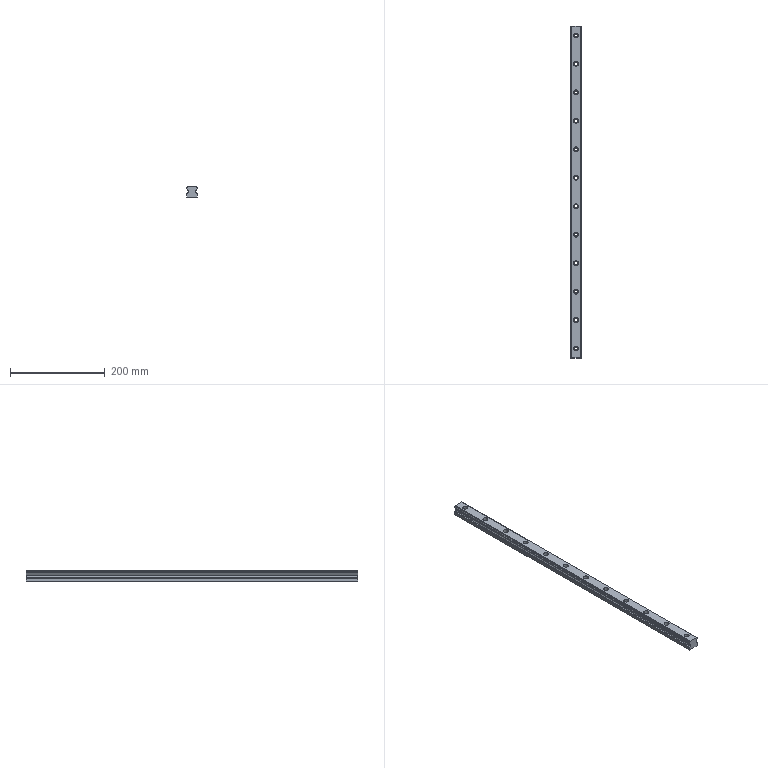Part | STEP file | Tube feed_id1570_x_t | 1 solid | 64 faces | box 23 x 700 x 22 mm | volume 297908 mm3 | cylinder 36 | plane 28 | commonest cylinder face diameters 6.5 x12 10.5 x12 3 x4 6 x4 1 x2 2 x2